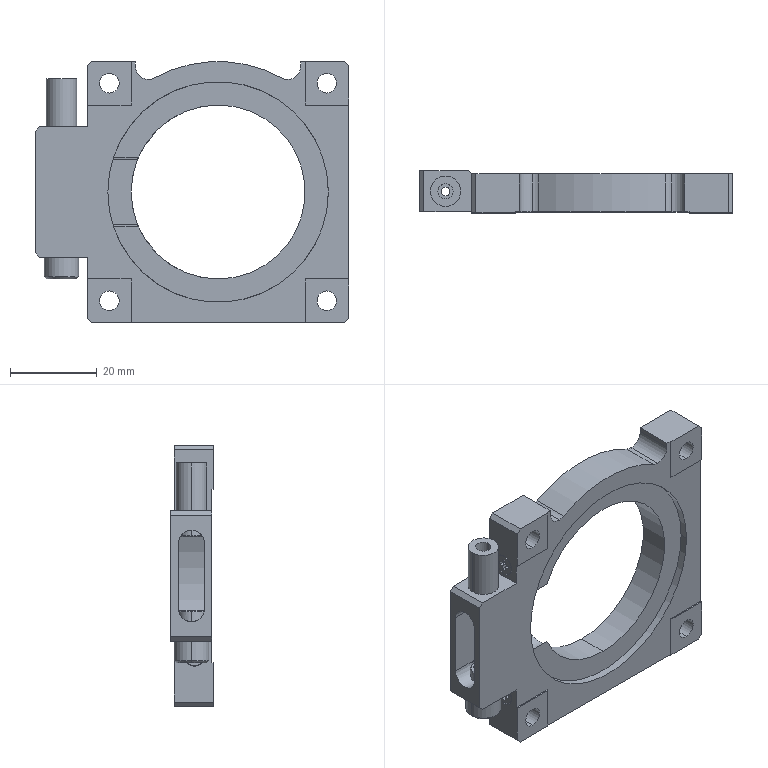Part | SolidWorks | features BaseBody 1 | 1 solid | 210 faces | box 72 x 9.75 x 60 mm | volume 18365 mm3 | plane 96 | cylinder 70 | cone 40 | spline 4 | commonest cylinder face diameters 6 x23 8 x10 4.5 x8 2.5 x4 2.9 x4 4.7 x4